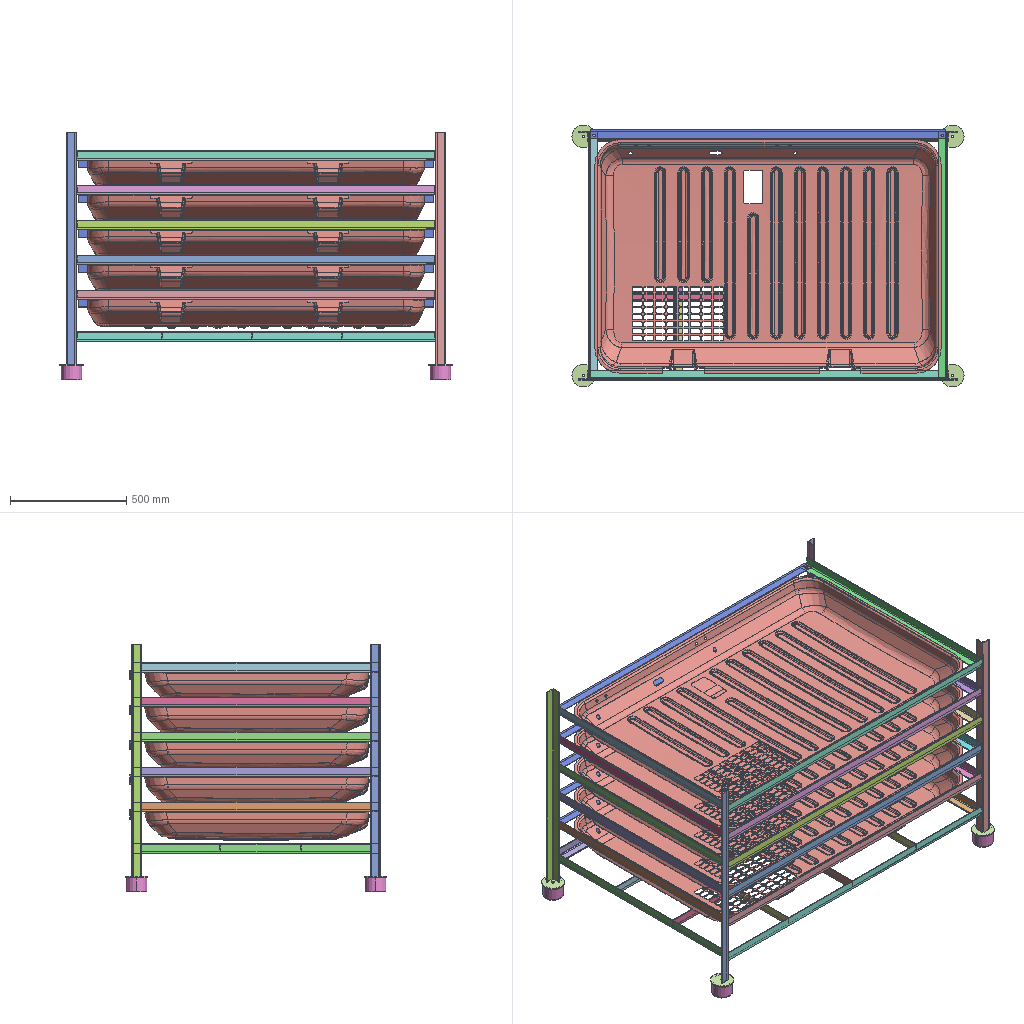Assembly | SolidWorks | 5 different items | 19 placed | box 1689 x 1128 x 1066 mm
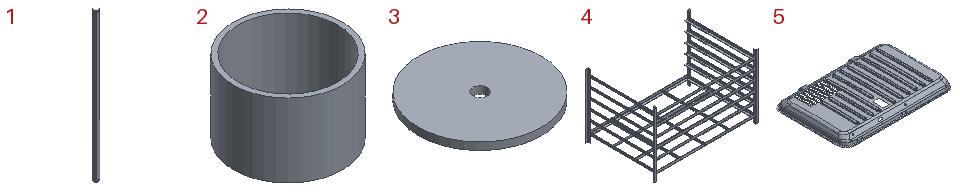Parts list (item | quantity | size | volume | features):
1 | x5 | 40 x 40 x 1530 mm | 360303 mm3 | features Cut 1, Extrusion 1
2 | x4 | 89 x 89 x 60 mm | 64088 mm3 | features Extrusion 1
3 | x4 | 100 x 100 x 6 mm | 46445 mm3 | features FlatPattern 1, SMBaseFlange 1, SheetMetal 1
4 | x1 | 1629 x 1070 x 1000 mm | 10278361 mm3 | features 3DProfileFeature 1, WeldMemberFeat 1, WeldmentFeature 1
5 | x5 | 1493 x 1007 x 129.32 mm | 2089478 mm3 | features MBimport 1
Mates (type | each side: item.copy, entity, surface, feature):
Coincident | 4.1 face plane GB/T9787-1988 hot-rolled equal-leg angle 40 X 4(1) | 5.1 face plane 2A5-54-32A10-OP10-DR-20241212-1216.stp
DistanceDim | 5.1 face plane 2A5-54-32A10-OP10-DR-20241212-1216.stp | 4.1 face plane GB/T9787-1988 hot-rolled equal-leg angle 40 X 4(1) | 2 times
Coincident | 4.1 face plane GB/T9787-1988 hot-rolled equal-leg angle 40 X 4(1) | 1.1 face plane Boss-Extrude1
DistanceDim | 4.1 face plane GB/T9787-1988 hot-rolled equal-leg angle 40 X 4(1) | 1.1 face plane Boss-Extrude1 | 2 times
Coincident | 4.1 face plane GB/T9787-1988 hot-rolled equal-leg angle 40 X 4(1) | 3.1 face plane Base-Flange1
DistanceDim | 3.1 face cylinder Base-Flange1 | 4.1 face plane GB/T9787-1988 hot-rolled equal-leg angle 40 X 4(1)
Parallel | 4.1 face plane GB/T9787-1988 hot-rolled equal-leg angle 40 X 4(1) | 3.1 plane
Concentric | 3.1 face cylinder Base-Flange1 | 2.1 face cylinder Boss-Extrude1
Coincident | 3.1 face plane Base-Flange1 | 2.1 face plane Boss-Extrude1
Parallel | 4.1 face plane GB/T9787-1988 hot-rolled equal-leg angle 40 X 4(1) | 2.1 plane
DistanceDim | 4.1 face plane GB/T9787-1988 hot-rolled equal-leg angle 40 X 4(1) | 3.1 face cylinder Base-Flange1